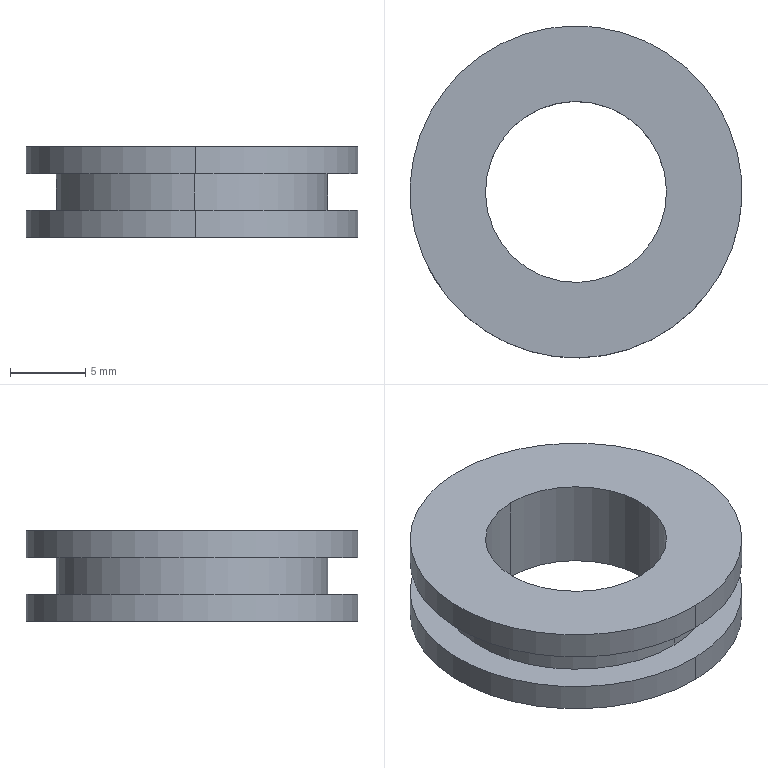Part | SolidWorks | features BaseBody 1 | 1 solid | 12 faces | box 22.001 x 22 x 6.003 mm | volume 1301 mm3 | cylinder 8 | plane 4 | commonest cylinder face diameters 22 x4 12 x2 18 x2
STEP:
#1=CARTESIAN_POINT('',(342.003,186.406,2.875));
#2=VERTEX_POINT('',#1);
#3=CARTESIAN_POINT('',(341.54,208.401,2.875));
#4=VERTEX_POINT('',#3);
#5=CARTESIAN_POINT('',(341.771,197.404,2.875));
#6=DIRECTION('',(-0.0001435,-0.000000521,1.));
#7=DIRECTION('',(1.,0.,0.0001435));
#8=AXIS2_PLACEMENT_3D('',#5,#6,#7);
#9=CIRCLE('',#8,11.);
#10=EDGE_CURVE('',#2,#4,#9,.T.);
#11=ORIENTED_EDGE('',*,*,#10,.F.);
#12=CARTESIAN_POINT('',(342.003,186.406,1.075));
#13=VERTEX_POINT('',#12);
#14=CARTESIAN_POINT('',(342.002,186.406,7.075));
#15=DIRECTION('',(0.0001435,0.000000521,-1.));
#16=VECTOR('',#15,1000.);
#17=LINE('',#14,#16);
#18=EDGE_CURVE('',#2,#13,#17,.T.);
#19=ORIENTED_EDGE('',*,*,#18,.T.);
#20=CARTESIAN_POINT('',(341.54,208.401,1.075));
#21=VERTEX_POINT('',#20);
#22=CARTESIAN_POINT('',(341.771,197.404,1.075));
#23=DIRECTION('',(0.0001435,0.000000521,-1.));
#24=DIRECTION('',(1.,0.,0.0001435));
#25=AXIS2_PLACEMENT_3D('',#22,#23,#24);
#26=CIRCLE('',#25,11.);
#27=EDGE_CURVE('',#21,#13,#26,.T.);
#28=ORIENTED_EDGE('',*,*,#27,.F.);
#29=CARTESIAN_POINT('',(341.539,208.401,7.075));
#30=DIRECTION('',(0.0001435,0.000000521,-1.));
#31=VECTOR('',#30,1000.);
#32=LINE('',#29,#31);
#33=EDGE_CURVE('',#4,#21,#32,.T.);
#34=ORIENTED_EDGE('',*,*,#33,.F.);
#35=EDGE_LOOP('',(#11,#19,#28,#34));
#36=FACE_OUTER_BOUND('',#35,.T.);
#37=CARTESIAN_POINT('',(341.771,197.404,7.075));
#38=DIRECTION('',(0.0001435,0.000000521,-1.));
#39=DIRECTION('',(-0.02104,0.9998,-0.000002497));
#40=AXIS2_PLACEMENT_3D('',#37,#38,#39);
#41=CYLINDRICAL_SURFACE('',#40,11.);
#42=ADVANCED_FACE('',(#36),#41,.T.);
#43=CARTESIAN_POINT('',(341.582,206.402,2.875));
#44=VERTEX_POINT('',#43);
#45=CARTESIAN_POINT('',(341.961,188.406,2.875));
#46=VERTEX_POINT('',#45);
#47=CARTESIAN_POINT('',(341.771,197.404,2.875));
#48=DIRECTION('',(0.0001435,0.000000521,-1.));
#49=DIRECTION('',(-0.02104,0.9998,-0.000002497));
#50=AXIS2_PLACEMENT_3D('',#47,#48,#49);
#51=CIRCLE('',#50,9.);
#52=EDGE_CURVE('',#44,#46,#51,.T.);
#53=ORIENTED_EDGE('',*,*,#52,.F.);
#54=CARTESIAN_POINT('',(341.582,206.402,5.275));
#55=VERTEX_POINT('',#54);
#56=CARTESIAN_POINT('',(341.582,206.402,1.075));
#57=DIRECTION('',(-0.0001435,-0.000000521,1.));
#58=VECTOR('',#57,1000.);
#59=LINE('',#56,#58);
#60=EDGE_CURVE('',#44,#55,#59,.T.);
#61=ORIENTED_EDGE('',*,*,#60,.T.);
#62=CARTESIAN_POINT('',(341.96,188.406,5.275));
#63=VERTEX_POINT('',#62);
#64=CARTESIAN_POINT('',(341.771,197.404,5.275));
#65=DIRECTION('',(-0.0001435,-0.000000521,1.));
#66=DIRECTION('',(-0.02104,0.9998,-0.000002497));
#67=AXIS2_PLACEMENT_3D('',#64,#65,#66);
#68=CIRCLE('',#67,9.);
#69=EDGE_CURVE('',#63,#55,#68,.T.);
#70=ORIENTED_EDGE('',*,*,#69,.F.);
#71=CARTESIAN_POINT('',(341.961,188.406,1.075));
#72=DIRECTION('',(-0.0001435,-0.000000521,1.));
#73=VECTOR('',#72,1000.);
#74=LINE('',#71,#73);
#75=EDGE_CURVE('',#46,#63,#74,.T.);
#76=ORIENTED_EDGE('',*,*,#75,.F.);
#77=EDGE_LOOP('',(#53,#61,#70,#76));
#78=FACE_OUTER_BOUND('',#77,.T.);
#79=CARTESIAN_POINT('',(341.771,197.404,1.075));
#80=DIRECTION('',(-0.0001435,-0.000000521,1.));
#81=DIRECTION('',(0.02104,-0.9998,0.000002497));
#82=AXIS2_PLACEMENT_3D('',#79,#80,#81);
#83=CYLINDRICAL_SURFACE('',#82,9.);
#84=ADVANCED_FACE('',(#78),#83,.T.);
#85=CARTESIAN_POINT('',(342.002,186.406,7.075));
#86=VERTEX_POINT('',#85);
#87=CARTESIAN_POINT('',(341.539,208.401,7.075));
#88=VERTEX_POINT('',#87);
#89=CARTESIAN_POINT('',(341.771,197.404,7.075));
#90=DIRECTION('',(-0.0001435,-0.000000521,1.));
#91=DIRECTION('',(-1.,0.,-0.0001435));
#92=AXIS2_PLACEMENT_3D('',#89,#90,#91);
#93=CIRCLE('',#92,11.);
#94=EDGE_CURVE('',#86,#88,#93,.T.);
#95=ORIENTED_EDGE('',*,*,#94,.F.);
#96=CARTESIAN_POINT('',(342.002,186.406,5.275));
#97=VERTEX_POINT('',#96);
#98=CARTESIAN_POINT('',(342.002,186.406,7.075));
#99=DIRECTION('',(0.0001435,0.000000521,-1.));
#100=VECTOR('',#99,1000.);
#101=LINE('',#98,#100);
#102=EDGE_CURVE('',#86,#97,#101,.T.);
#103=ORIENTED_EDGE('',*,*,#102,.T.);
#104=CARTESIAN_POINT('',(341.539,208.401,5.275));
#105=VERTEX_POINT('',#104);
#106=CARTESIAN_POINT('',(341.771,197.404,5.275));
#107=DIRECTION('',(0.0001435,0.000000521,-1.));
#108=DIRECTION('',(-0.02104,0.9998,-0.000002497));
#109=AXIS2_PLACEMENT_3D('',#106,#107,#108);
#110=CIRCLE('',#109,11.);
#111=EDGE_CURVE('',#105,#97,#110,.T.);
#112=ORIENTED_EDGE('',*,*,#111,.F.);
#113=CARTESIAN_POINT('',(341.539,208.401,7.075));
#114=DIRECTION('',(0.0001435,0.000000521,-1.));
#115=VECTOR('',#114,1000.);
#116=LINE('',#113,#115);
#117=EDGE_CURVE('',#88,#105,#116,.T.);
#118=ORIENTED_EDGE('',*,*,#117,.F.);
#119=EDGE_LOOP('',(#95,#103,#112,#118));
#120=FACE_OUTER_BOUND('',#119,.T.);
#121=CARTESIAN_POINT('',(341.771,197.404,7.075));
#122=DIRECTION('',(0.0001435,0.000000521,-1.));
#123=DIRECTION('',(-0.02104,0.9998,-0.000002497));
#124=AXIS2_PLACEMENT_3D('',#121,#122,#123);
#125=CYLINDRICAL_SURFACE('',#124,11.);
#126=ADVANCED_FACE('',(#120),#125,.T.);
#127=CARTESIAN_POINT('',(341.645,203.402,1.075));
#128=VERTEX_POINT('',#127);
#129=CARTESIAN_POINT('',(341.898,191.405,1.075));
#130=VERTEX_POINT('',#129);
#131=CARTESIAN_POINT('',(341.771,197.404,1.075));
#132=DIRECTION('',(-0.0001435,-0.000000521,1.));
#133=DIRECTION('',(-0.02104,0.9998,-0.000002497));
#134=AXIS2_PLACEMENT_3D('',#131,#132,#133);
#135=CIRCLE('',#134,6.);
#136=EDGE_CURVE('',#128,#130,#135,.T.);
#137=ORIENTED_EDGE('',*,*,#136,.F.);
#138=CARTESIAN_POINT('',(341.644,203.402,7.075));
#139=VERTEX_POINT('',#138);
#140=CARTESIAN_POINT('',(341.645,203.402,1.075));
#141=DIRECTION('',(-0.0001435,-0.000000521,1.));
#142=VECTOR('',#141,1000.);
#143=LINE('',#140,#142);
#144=EDGE_CURVE('',#128,#139,#143,.T.);
#145=ORIENTED_EDGE('',*,*,#144,.T.);
#146=CARTESIAN_POINT('',(341.897,191.405,7.075));
#147=VERTEX_POINT('',#146);
#148=CARTESIAN_POINT('',(341.771,197.404,7.075));
#149=DIRECTION('',(0.0001435,0.000000521,-1.));
#150=DIRECTION('',(-0.02104,0.9998,-0.000002497));
#151=AXIS2_PLACEMENT_3D('',#148,#149,#150);
#152=CIRCLE('',#151,6.);
#153=EDGE_CURVE('',#147,#139,#152,.T.);
#154=ORIENTED_EDGE('',*,*,#153,.F.);
#155=CARTESIAN_POINT('',(341.898,191.405,1.075));
#156=DIRECTION('',(-0.0001435,-0.000000521,1.));
#157=VECTOR('',#156,1000.);
#158=LINE('',#155,#157);
#159=EDGE_CURVE('',#130,#147,#158,.T.);
#160=ORIENTED_EDGE('',*,*,#159,.F.);
#161=EDGE_LOOP('',(#137,#145,#154,#160));
#162=FACE_OUTER_BOUND('',#161,.T.);
#163=CARTESIAN_POINT('',(341.771,197.404,1.075));
#164=DIRECTION('',(-0.0001435,-0.000000521,1.));
#165=DIRECTION('',(0.02104,-0.9998,0.000002497));
#166=AXIS2_PLACEMENT_3D('',#163,#164,#165);
#167=CYLINDRICAL_SURFACE('',#166,6.);
#168=ADVANCED_FACE('',(#162),#167,.F.);
#169=CARTESIAN_POINT('',(341.771,197.404,1.075));
#170=DIRECTION('',(-0.0001435,-0.000000521,1.));
#171=DIRECTION('',(-0.02104,0.9998,-0.000002497));
#172=AXIS2_PLACEMENT_3D('',#169,#170,#171);
#173=CIRCLE('',#172,6.);
#174=EDGE_CURVE('',#130,#128,#173,.T.);
#175=ORIENTED_EDGE('',*,*,#174,.T.);
#176=ORIENTED_EDGE('',*,*,#136,.T.);
#177=EDGE_LOOP('',(#175,#176));
#178=FACE_BOUND('',#177,.T.);
#179=ORIENTED_EDGE('',*,*,#27,.T.);
#180=CARTESIAN_POINT('',(341.771,197.404,1.075));
#181=DIRECTION('',(0.0001435,0.000000521,-1.));
#182=DIRECTION('',(1.,0.,0.0001435));
#183=AXIS2_PLACEMENT_3D('',#180,#181,#182);
#184=CIRCLE('',#183,11.);
#185=EDGE_CURVE('',#13,#21,#184,.T.);
#186=ORIENTED_EDGE('',*,*,#185,.T.);
#187=EDGE_LOOP('',(#179,#186));
#188=FACE_OUTER_BOUND('',#187,.T.);
#189=CARTESIAN_POINT('',(341.771,197.404,1.075));
#190=DIRECTION('',(0.0001435,0.000000521,-1.));
#191=DIRECTION('',(0.,-1.,-0.000000521));
#192=AXIS2_PLACEMENT_3D('',#189,#190,#191);
#193=PLANE('',#192);
#194=ADVANCED_FACE('',(#178,#188),#193,.T.);
#195=ORIENTED_EDGE('',*,*,#144,.F.);
#196=ORIENTED_EDGE('',*,*,#174,.F.);
#197=ORIENTED_EDGE('',*,*,#159,.T.);
#198=CARTESIAN_POINT('',(341.771,197.404,7.075));
#199=DIRECTION('',(0.0001435,0.000000521,-1.));
#200=DIRECTION('',(-0.02104,0.9998,-0.000002497));
#201=AXIS2_PLACEMENT_3D('',#198,#199,#200);
#202=CIRCLE('',#201,6.);
#203=EDGE_CURVE('',#139,#147,#202,.T.);
#204=ORIENTED_EDGE('',*,*,#203,.F.);
#205=EDGE_LOOP('',(#195,#196,#197,#204));
#206=FACE_OUTER_BOUND('',#205,.T.);
#207=CARTESIAN_POINT('',(341.771,197.404,1.075));
#208=DIRECTION('',(-0.0001435,-0.000000521,1.));
#209=DIRECTION('',(0.02104,-0.9998,0.000002497));
#210=AXIS2_PLACEMENT_3D('',#207,#208,#209);
#211=CYLINDRICAL_SURFACE('',#210,6.);
#212=ADVANCED_FACE('',(#206),#211,.F.);
#213=ORIENTED_EDGE('',*,*,#153,.T.);
#214=ORIENTED_EDGE('',*,*,#203,.T.);
#215=EDGE_LOOP('',(#213,#214));
#216=FACE_BOUND('',#215,.T.);
#217=CARTESIAN_POINT('',(341.771,197.404,7.075));
#218=DIRECTION('',(-0.0001435,-0.000000521,1.));
#219=DIRECTION('',(-1.,0.,-0.0001435));
#220=AXIS2_PLACEMENT_3D('',#217,#218,#219);
#221=CIRCLE('',#220,11.);
#222=EDGE_CURVE('',#88,#86,#221,.T.);
#223=ORIENTED_EDGE('',*,*,#222,.T.);
#224=ORIENTED_EDGE('',*,*,#94,.T.);
#225=EDGE_LOOP('',(#223,#224));
#226=FACE_OUTER_BOUND('',#225,.T.);
#227=CARTESIAN_POINT('',(341.771,197.404,7.075));
#228=DIRECTION('',(-0.0001435,-0.000000521,1.));
#229=DIRECTION('',(-0.003633,1.,0.));
#230=AXIS2_PLACEMENT_3D('',#227,#228,#229);
#231=PLANE('',#230);
#232=ADVANCED_FACE('',(#216,#226),#231,.T.);
#233=ORIENTED_EDGE('',*,*,#102,.F.);
#234=ORIENTED_EDGE('',*,*,#222,.F.);
#235=ORIENTED_EDGE('',*,*,#117,.T.);
#236=CARTESIAN_POINT('',(341.771,197.404,5.275));
#237=DIRECTION('',(0.0001435,0.000000521,-1.));
#238=DIRECTION('',(-0.02104,0.9998,-0.000002497));
#239=AXIS2_PLACEMENT_3D('',#236,#237,#238);
#240=CIRCLE('',#239,11.);
#241=EDGE_CURVE('',#97,#105,#240,.T.);
#242=ORIENTED_EDGE('',*,*,#241,.F.);
#243=EDGE_LOOP('',(#233,#234,#235,#242));
#244=FACE_OUTER_BOUND('',#243,.T.);
#245=CARTESIAN_POINT('',(341.771,197.404,7.075));
#246=DIRECTION('',(0.0001435,0.000000521,-1.));
#247=DIRECTION('',(-0.02104,0.9998,-0.000002497));
#248=AXIS2_PLACEMENT_3D('',#245,#246,#247);
#249=CYLINDRICAL_SURFACE('',#248,11.);
#250=ADVANCED_FACE('',(#244),#249,.T.);
#251=ORIENTED_EDGE('',*,*,#69,.T.);
#252=CARTESIAN_POINT('',(341.771,197.404,5.275));
#253=DIRECTION('',(-0.0001435,-0.000000521,1.));
#254=DIRECTION('',(-0.02104,0.9998,-0.000002497));
#255=AXIS2_PLACEMENT_3D('',#252,#253,#254);
#256=CIRCLE('',#255,9.);
#257=EDGE_CURVE('',#55,#63,#256,.T.);
#258=ORIENTED_EDGE('',*,*,#257,.T.);
#259=EDGE_LOOP('',(#251,#258));
#260=FACE_BOUND('',#259,.T.);
#261=ORIENTED_EDGE('',*,*,#111,.T.);
#262=ORIENTED_EDGE('',*,*,#241,.T.);
#263=EDGE_LOOP('',(#261,#262));
#264=FACE_OUTER_BOUND('',#263,.T.);
#265=CARTESIAN_POINT('',(341.771,197.404,5.275));
#266=DIRECTION('',(-0.0001435,-0.000000521,1.));
#267=DIRECTION('',(-0.003633,1.,0.));
#268=AXIS2_PLACEMENT_3D('',#265,#266,#267);
#269=PLANE('',#268);
#270=ADVANCED_FACE('',(#260,#264),#269,.F.);
#271=ORIENTED_EDGE('',*,*,#60,.F.);
#272=CARTESIAN_POINT('',(341.771,197.404,2.875));
#273=DIRECTION('',(0.0001435,0.000000521,-1.));
#274=DIRECTION('',(-0.02104,0.9998,-0.000002497));
#275=AXIS2_PLACEMENT_3D('',#272,#273,#274);
#276=CIRCLE('',#275,9.);
#277=EDGE_CURVE('',#46,#44,#276,.T.);
#278=ORIENTED_EDGE('',*,*,#277,.F.);
#279=ORIENTED_EDGE('',*,*,#75,.T.);
#280=ORIENTED_EDGE('',*,*,#257,.F.);
#281=EDGE_LOOP('',(#271,#278,#279,#280));
#282=FACE_OUTER_BOUND('',#281,.T.);
#283=CARTESIAN_POINT('',(341.771,197.404,1.075));
#284=DIRECTION('',(-0.0001435,-0.000000521,1.));
#285=DIRECTION('',(0.02104,-0.9998,0.000002497));
#286=AXIS2_PLACEMENT_3D('',#283,#284,#285);
#287=CYLINDRICAL_SURFACE('',#286,9.);
#288=ADVANCED_FACE('',(#282),#287,.T.);
#289=ORIENTED_EDGE('',*,*,#277,.T.);
#290=ORIENTED_EDGE('',*,*,#52,.T.);
#291=EDGE_LOOP('',(#289,#290));
#292=FACE_BOUND('',#291,.T.);
#293=CARTESIAN_POINT('',(341.771,197.404,2.875));
#294=DIRECTION('',(-0.0001435,-0.000000521,1.));
#295=DIRECTION('',(1.,0.,0.0001435));
#296=AXIS2_PLACEMENT_3D('',#293,#294,#295);
#297=CIRCLE('',#296,11.);
#298=EDGE_CURVE('',#4,#2,#297,.T.);
#299=ORIENTED_EDGE('',*,*,#298,.T.);
#300=ORIENTED_EDGE('',*,*,#10,.T.);
#301=EDGE_LOOP('',(#299,#300));
#302=FACE_OUTER_BOUND('',#301,.T.);
#303=CARTESIAN_POINT('',(341.771,197.404,2.875));
#304=DIRECTION('',(0.0001435,0.000000521,-1.));
#305=DIRECTION('',(0.,-1.,-0.000000521));
#306=AXIS2_PLACEMENT_3D('',#303,#304,#305);
#307=PLANE('',#306);
#308=ADVANCED_FACE('',(#292,#302),#307,.F.);
#309=ORIENTED_EDGE('',*,*,#18,.F.);
#310=ORIENTED_EDGE('',*,*,#298,.F.);
#311=ORIENTED_EDGE('',*,*,#33,.T.);
#312=ORIENTED_EDGE('',*,*,#185,.F.);
#313=EDGE_LOOP('',(#309,#310,#311,#312));
#314=FACE_OUTER_BOUND('',#313,.T.);
#315=CARTESIAN_POINT('',(341.771,197.404,7.075));
#316=DIRECTION('',(0.0001435,0.000000521,-1.));
#317=DIRECTION('',(-0.02104,0.9998,-0.000002497));
#318=AXIS2_PLACEMENT_3D('',#315,#316,#317);
#319=CYLINDRICAL_SURFACE('',#318,11.);
#320=ADVANCED_FACE('',(#314),#319,.T.);
#321=CLOSED_SHELL('',(#42,#84,#126,#168,#194,#212,#232,#250,#270,#288,#308,#320));
#322=MANIFOLD_SOLID_BREP('',#321);
#323=CARTESIAN_POINT('',(0.,0.,0.));
#324=DIRECTION('',(0.,0.,1.));
#325=DIRECTION('',(1.,0.,0.));
#326=AXIS2_PLACEMENT_3D('',#323,#324,#325);
#327=(LENGTH_UNIT()NAMED_UNIT(*)SI_UNIT(.MILLI.,.METRE.));
#328=UNCERTAINTY_MEASURE_WITH_UNIT(LENGTH_MEASURE(0.00001),#327,'','');
#329=(NAMED_UNIT(*)PLANE_ANGLE_UNIT()SI_UNIT($,.RADIAN.));
#330=(NAMED_UNIT(*)SI_UNIT($,.STERADIAN.)SOLID_ANGLE_UNIT());
#331=(GEOMETRIC_REPRESENTATION_CONTEXT(3)GLOBAL_UNCERTAINTY_ASSIGNED_CONTEXT((#328))GLOBAL_UNIT_ASSIGNED_CONTEXT((#327,#329,#330))REPRESENTATION_CONTEXT('',''));
#332=ADVANCED_BREP_SHAPE_REPRESENTATION('',(#322,#326),#331);